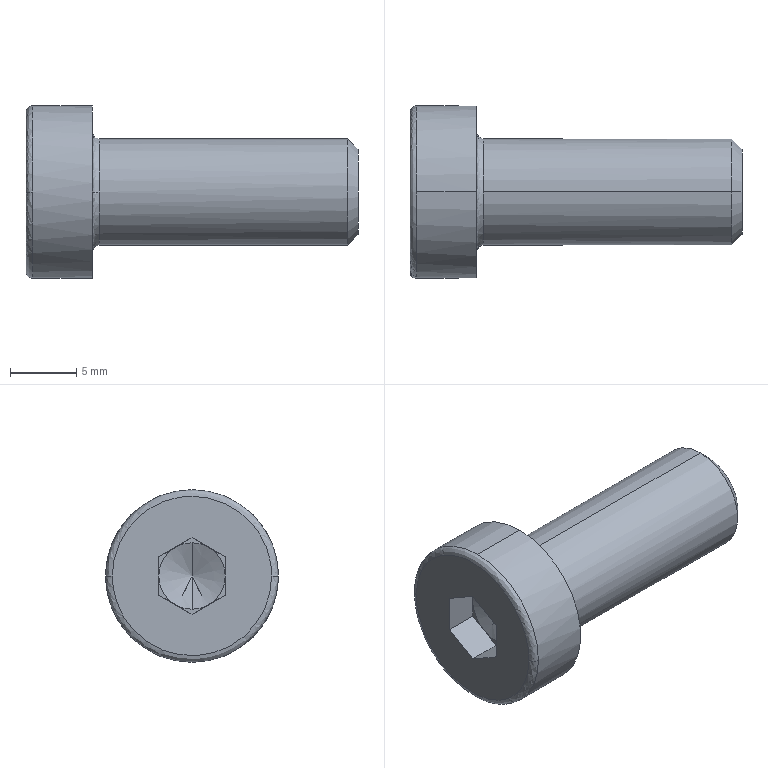Part | SolidWorks | features BaseBody 1 | 1 solid | 27 faces | box 25 x 13 x 13 mm | volume 1601 mm3 | plane 15 | spline 4 | cylinder 4 | cone 4 | commonest cylinder face diameters 8 x2 13 x2
STEP:
#1=CARTESIAN_POINT('',(-16.5,4.,0.));
#2=VERTEX_POINT('',#1);
#3=CARTESIAN_POINT('',(-16.5,0.,4.));
#4=VERTEX_POINT('',#3);
#5=CARTESIAN_POINT('',(-16.5,0.,0.));
#6=DIRECTION('',(1.,0.,0.));
#7=DIRECTION('',(0.,0.,-1.));
#8=AXIS2_PLACEMENT_3D('',#5,#6,#7);
#9=CIRCLE('',#8,4.);
#10=EDGE_CURVE('',#2,#4,#9,.T.);
#11=ORIENTED_EDGE('',*,*,#10,.F.);
#12=CARTESIAN_POINT('',(-17.,4.5,0.));
#13=VERTEX_POINT('',#12);
#14=CARTESIAN_POINT('',(-16.5,4.5,0.));
#15=DIRECTION('',(0.,0.,-1.));
#16=DIRECTION('',(0.,1.,0.));
#17=AXIS2_PLACEMENT_3D('',#14,#15,#16);
#18=CIRCLE('',#17,0.5);
#19=EDGE_CURVE('',#2,#13,#18,.T.);
#20=ORIENTED_EDGE('',*,*,#19,.T.);
#21=CARTESIAN_POINT('',(-17.,0.,4.5));
#22=VERTEX_POINT('',#21);
#23=CARTESIAN_POINT('',(-17.,0.,4.5));
#24=CARTESIAN_POINT('',(-17.,0.286,4.5));
#25=CARTESIAN_POINT('',(-17.,0.7076,4.461));
#26=CARTESIAN_POINT('',(-17.,1.186,4.345));
#27=CARTESIAN_POINT('',(-17.,1.422,4.27));
#28=CARTESIAN_POINT('',(-17.,1.523,4.235));
#29=CARTESIAN_POINT('',(-17.,1.59,4.21));
#30=CARTESIAN_POINT('',(-17.,1.621,4.198));
#31=CARTESIAN_POINT('',(-17.,1.798,4.128));
#32=CARTESIAN_POINT('',(-17.,2.004,4.034));
#33=CARTESIAN_POINT('',(-17.,2.203,3.925));
#34=CARTESIAN_POINT('',(-17.,2.334,3.848));
#35=CARTESIAN_POINT('',(-17.,2.398,3.809));
#36=CARTESIAN_POINT('',(-17.,2.722,3.597));
#37=CARTESIAN_POINT('',(-17.,2.963,3.401));
#38=CARTESIAN_POINT('',(-17.,3.292,3.072));
#39=CARTESIAN_POINT('',(-17.,3.447,2.9));
#40=CARTESIAN_POINT('',(-17.,3.589,2.716));
#41=CARTESIAN_POINT('',(-17.,3.68,2.591));
#42=CARTESIAN_POINT('',(-17.,3.725,2.526));
#43=CARTESIAN_POINT('',(-17.,3.85,2.335));
#44=CARTESIAN_POINT('',(-17.,3.964,2.139));
#45=CARTESIAN_POINT('',(-17.,4.08,1.901));
#46=CARTESIAN_POINT('',(-17.,4.134,1.779));
#47=CARTESIAN_POINT('',(-17.,4.155,1.727));
#48=CARTESIAN_POINT('',(-17.,4.17,1.692));
#49=CARTESIAN_POINT('',(-17.,4.177,1.673));
#50=CARTESIAN_POINT('',(-17.,4.395,1.125));
#51=CARTESIAN_POINT('',(-17.,4.5,0.5724));
#52=CARTESIAN_POINT('',(-17.,4.5,0.));
#53=B_SPLINE_CURVE_WITH_KNOTS('',3,(#23,#24,#25,#26,#27,#28,#29,#30,#31,#32,#33,#34,#35,#36,#37,#38,#39,#40,#41,#42,#43,#44,#45,#46,#47,#48,#49,#50,#51,#52),.UNSPECIFIED.,.F.,.F.,(4,1,1,1,2,2,1,2,2,2,1,2,2,1,1,1,2,2,4),(0.,0.125,0.1875,0.2187,0.2344,0.25,0.3125,0.3438,0.375,0.5,0.5625,0.5938,0.625,0.6875,0.7188,0.7344,0.7422,0.75,1.),.UNSPECIFIED.);
#54=EDGE_CURVE('',#22,#13,#53,.T.);
#55=ORIENTED_EDGE('',*,*,#54,.F.);
#56=CARTESIAN_POINT('',(-17.,-4.5,0.));
#57=VERTEX_POINT('',#56);
#58=CARTESIAN_POINT('',(-17.,-4.5,0.));
#59=CARTESIAN_POINT('',(-17.,-4.5,0.286));
#60=CARTESIAN_POINT('',(-17.,-4.461,0.7076));
#61=CARTESIAN_POINT('',(-17.,-4.345,1.186));
#62=CARTESIAN_POINT('',(-17.,-4.27,1.422));
#63=CARTESIAN_POINT('',(-17.,-4.235,1.523));
#64=CARTESIAN_POINT('',(-17.,-4.21,1.59));
#65=CARTESIAN_POINT('',(-17.,-4.198,1.621));
#66=CARTESIAN_POINT('',(-17.,-4.128,1.798));
#67=CARTESIAN_POINT('',(-17.,-4.034,2.004));
#68=CARTESIAN_POINT('',(-17.,-3.925,2.203));
#69=CARTESIAN_POINT('',(-17.,-3.848,2.334));
#70=CARTESIAN_POINT('',(-17.,-3.809,2.398));
#71=CARTESIAN_POINT('',(-17.,-3.597,2.722));
#72=CARTESIAN_POINT('',(-17.,-3.401,2.963));
#73=CARTESIAN_POINT('',(-17.,-3.072,3.292));
#74=CARTESIAN_POINT('',(-17.,-2.9,3.447));
#75=CARTESIAN_POINT('',(-17.,-2.716,3.589));
#76=CARTESIAN_POINT('',(-17.,-2.591,3.68));
#77=CARTESIAN_POINT('',(-17.,-2.526,3.725));
#78=CARTESIAN_POINT('',(-17.,-2.335,3.85));
#79=CARTESIAN_POINT('',(-17.,-2.139,3.964));
#80=CARTESIAN_POINT('',(-17.,-1.901,4.08));
#81=CARTESIAN_POINT('',(-17.,-1.779,4.134));
#82=CARTESIAN_POINT('',(-17.,-1.727,4.155));
#83=CARTESIAN_POINT('',(-17.,-1.692,4.17));
#84=CARTESIAN_POINT('',(-17.,-1.673,4.177));
#85=CARTESIAN_POINT('',(-17.,-1.125,4.395));
#86=CARTESIAN_POINT('',(-17.,-0.5724,4.5));
#87=CARTESIAN_POINT('',(-17.,0.,4.5));
#88=B_SPLINE_CURVE_WITH_KNOTS('',3,(#58,#59,#60,#61,#62,#63,#64,#65,#66,#67,#68,#69,#70,#71,#72,#73,#74,#75,#76,#77,#78,#79,#80,#81,#82,#83,#84,#85,#86,#87),.UNSPECIFIED.,.F.,.F.,(4,1,1,1,2,2,1,2,2,2,1,2,2,1,1,1,2,2,4),(0.,0.125,0.1875,0.2188,0.2344,0.25,0.3125,0.3438,0.375,0.5,0.5625,0.5938,0.625,0.6875,0.7188,0.7344,0.7422,0.75,1.),.UNSPECIFIED.);
#89=EDGE_CURVE('',#57,#22,#88,.T.);
#90=ORIENTED_EDGE('',*,*,#89,.F.);
#91=CARTESIAN_POINT('',(-16.5,-4.,0.));
#92=VERTEX_POINT('',#91);
#93=CARTESIAN_POINT('',(-16.5,-4.5,0.));
#94=DIRECTION('',(0.,0.,1.));
#95=DIRECTION('',(0.,-1.,0.));
#96=AXIS2_PLACEMENT_3D('',#93,#94,#95);
#97=CIRCLE('',#96,0.5);
#98=EDGE_CURVE('',#92,#57,#97,.T.);
#99=ORIENTED_EDGE('',*,*,#98,.F.);
#100=CARTESIAN_POINT('',(-16.5,0.,0.));
#101=DIRECTION('',(1.,0.,0.));
#102=DIRECTION('',(0.,0.,-1.));
#103=AXIS2_PLACEMENT_3D('',#100,#101,#102);
#104=CIRCLE('',#103,4.);
#105=EDGE_CURVE('',#4,#92,#104,.T.);
#106=ORIENTED_EDGE('',*,*,#105,.F.);
#107=EDGE_LOOP('',(#11,#20,#55,#90,#99,#106));
#108=FACE_OUTER_BOUND('',#107,.T.);
#109=CARTESIAN_POINT('',(-16.5,-4.,0.));
#110=CARTESIAN_POINT('',(-16.5,-4.,8.));
#111=CARTESIAN_POINT('',(-16.5,4.,8.));
#112=CARTESIAN_POINT('',(-16.5,4.,0.));
#113=CARTESIAN_POINT('',(-16.793,-4.,0.));
#114=CARTESIAN_POINT('',(-16.793,-4.,8.));
#115=CARTESIAN_POINT('',(-16.793,4.,8.));
#116=CARTESIAN_POINT('',(-16.793,4.,0.));
#117=CARTESIAN_POINT('',(-17.,-4.207,0.));
#118=CARTESIAN_POINT('',(-17.,-4.207,8.414));
#119=CARTESIAN_POINT('',(-17.,4.207,8.414));
#120=CARTESIAN_POINT('',(-17.,4.207,0.));
#121=CARTESIAN_POINT('',(-17.,-4.5,0.));
#122=CARTESIAN_POINT('',(-17.,-4.5,9.));
#123=CARTESIAN_POINT('',(-17.,4.5,9.));
#124=CARTESIAN_POINT('',(-17.,4.5,0.));
#125=(BOUNDED_SURFACE()B_SPLINE_SURFACE(3,3,((#109,#110,#111,#112),(#113,#114,#115,#116),(#117,#118,#119,#120),(#121,#122,#123,#124)),.UNSPECIFIED.,.F.,.F.,.T.)B_SPLINE_SURFACE_WITH_KNOTS((4,4),(4,4),(0.,1.),(0.,1.),.UNSPECIFIED.)GEOMETRIC_REPRESENTATION_ITEM()RATIONAL_B_SPLINE_SURFACE(((1.,0.3333,0.3333,1.),(0.8047,0.2682,0.2682,0.8047),(0.8047,0.2682,0.2682,0.8047),(1.,0.3333,0.3333,1.)))REPRESENTATION_ITEM('')SURFACE());
#126=ADVANCED_FACE('',(#108),#125,.F.);
#127=CARTESIAN_POINT('',(-22.,-6.,0.));
#128=VERTEX_POINT('',#127);
#129=CARTESIAN_POINT('',(-22.,6.,0.));
#130=VERTEX_POINT('',#129);
#131=CARTESIAN_POINT('',(-22.,-6.,0.));
#132=CARTESIAN_POINT('',(-22.,-6.,-12.));
#133=CARTESIAN_POINT('',(-22.,6.,-12.));
#134=CARTESIAN_POINT('',(-22.,6.,0.));
#135=(BOUNDED_CURVE()B_SPLINE_CURVE(3,(#131,#132,#133,#134),.UNSPECIFIED.,.F.,.T.)B_SPLINE_CURVE_WITH_KNOTS((4,4),(0.,1.),.UNSPECIFIED.)CURVE()GEOMETRIC_REPRESENTATION_ITEM()RATIONAL_B_SPLINE_CURVE((1.,0.3333,0.3333,1.))REPRESENTATION_ITEM(''));
#136=EDGE_CURVE('',#128,#130,#135,.T.);
#137=ORIENTED_EDGE('',*,*,#136,.T.);
#138=CARTESIAN_POINT('',(-21.5,6.5,0.));
#139=VERTEX_POINT('',#138);
#140=CARTESIAN_POINT('',(-21.5,6.,0.));
#141=DIRECTION('',(0.,0.,-1.));
#142=DIRECTION('',(0.,1.,0.));
#143=AXIS2_PLACEMENT_3D('',#140,#141,#142);
#144=CIRCLE('',#143,0.5);
#145=EDGE_CURVE('',#130,#139,#144,.T.);
#146=ORIENTED_EDGE('',*,*,#145,.T.);
#147=CARTESIAN_POINT('',(-21.5,0.,-6.5));
#148=VERTEX_POINT('',#147);
#149=CARTESIAN_POINT('',(-21.5,0.,0.));
#150=DIRECTION('',(1.,0.,0.));
#151=DIRECTION('',(0.,0.,-1.));
#152=AXIS2_PLACEMENT_3D('',#149,#150,#151);
#153=CIRCLE('',#152,6.5);
#154=EDGE_CURVE('',#148,#139,#153,.T.);
#155=ORIENTED_EDGE('',*,*,#154,.F.);
#156=CARTESIAN_POINT('',(-21.5,-6.5,0.));
#157=VERTEX_POINT('',#156);
#158=CARTESIAN_POINT('',(-21.5,0.,0.));
#159=DIRECTION('',(1.,0.,0.));
#160=DIRECTION('',(0.,0.,-1.));
#161=AXIS2_PLACEMENT_3D('',#158,#159,#160);
#162=CIRCLE('',#161,6.5);
#163=EDGE_CURVE('',#157,#148,#162,.T.);
#164=ORIENTED_EDGE('',*,*,#163,.F.);
#165=CARTESIAN_POINT('',(-21.5,-6.,0.));
#166=DIRECTION('',(0.,0.,1.));
#167=DIRECTION('',(0.,-1.,0.));
#168=AXIS2_PLACEMENT_3D('',#165,#166,#167);
#169=CIRCLE('',#168,0.5);
#170=EDGE_CURVE('',#128,#157,#169,.T.);
#171=ORIENTED_EDGE('',*,*,#170,.F.);
#172=EDGE_LOOP('',(#137,#146,#155,#164,#171));
#173=FACE_OUTER_BOUND('',#172,.T.);
#174=CARTESIAN_POINT('',(-22.,6.,0.));
#175=CARTESIAN_POINT('',(-22.,6.,-12.));
#176=CARTESIAN_POINT('',(-22.,-6.,-12.));
#177=CARTESIAN_POINT('',(-22.,-6.,0.));
#178=CARTESIAN_POINT('',(-22.,6.293,0.));
#179=CARTESIAN_POINT('',(-22.,6.293,-12.586));
#180=CARTESIAN_POINT('',(-22.,-6.293,-12.586));
#181=CARTESIAN_POINT('',(-22.,-6.293,0.));
#182=CARTESIAN_POINT('',(-21.793,6.5,0.));
#183=CARTESIAN_POINT('',(-21.793,6.5,-13.));
#184=CARTESIAN_POINT('',(-21.793,-6.5,-13.));
#185=CARTESIAN_POINT('',(-21.793,-6.5,0.));
#186=CARTESIAN_POINT('',(-21.5,6.5,0.));
#187=CARTESIAN_POINT('',(-21.5,6.5,-13.));
#188=CARTESIAN_POINT('',(-21.5,-6.5,-13.));
#189=CARTESIAN_POINT('',(-21.5,-6.5,0.));
#190=(BOUNDED_SURFACE()B_SPLINE_SURFACE(3,3,((#174,#175,#176,#177),(#178,#179,#180,#181),(#182,#183,#184,#185),(#186,#187,#188,#189)),.UNSPECIFIED.,.F.,.F.,.F.)B_SPLINE_SURFACE_WITH_KNOTS((4,4),(4,4),(0.,1.),(0.,1.),.UNSPECIFIED.)GEOMETRIC_REPRESENTATION_ITEM()RATIONAL_B_SPLINE_SURFACE(((1.,0.3333,0.3333,1.),(0.8047,0.2682,0.2682,0.8047),(0.8047,0.2682,0.2682,0.8047),(1.,0.3333,0.3333,1.)))REPRESENTATION_ITEM('')SURFACE());
#191=ADVANCED_FACE('',(#173),#190,.T.);
#192=CARTESIAN_POINT('',(-16.5,0.,-4.));
#193=VERTEX_POINT('',#192);
#194=CARTESIAN_POINT('',(-16.5,0.,0.));
#195=DIRECTION('',(1.,0.,0.));
#196=DIRECTION('',(0.,0.,-1.));
#197=AXIS2_PLACEMENT_3D('',#194,#195,#196);
#198=CIRCLE('',#197,4.);
#199=EDGE_CURVE('',#193,#2,#198,.T.);
#200=ORIENTED_EDGE('',*,*,#199,.T.);
#201=ORIENTED_EDGE('',*,*,#10,.T.);
#202=CARTESIAN_POINT('',(2.233,0.,4.));
#203=VERTEX_POINT('',#202);
#204=CARTESIAN_POINT('',(-7.133,0.,4.));
#205=DIRECTION('',(1.,0.,0.));
#206=VECTOR('',#205,1000.);
#207=LINE('',#204,#206);
#208=EDGE_CURVE('',#4,#203,#207,.T.);
#209=ORIENTED_EDGE('',*,*,#208,.T.);
#210=CARTESIAN_POINT('',(2.233,0.,-4.));
#211=VERTEX_POINT('',#210);
#212=CARTESIAN_POINT('',(2.233,0.,0.));
#213=DIRECTION('',(-1.,0.,0.));
#214=DIRECTION('',(0.,0.,-1.));
#215=AXIS2_PLACEMENT_3D('',#212,#213,#214);
#216=CIRCLE('',#215,4.);
#217=EDGE_CURVE('',#203,#211,#216,.T.);
#218=ORIENTED_EDGE('',*,*,#217,.T.);
#219=CARTESIAN_POINT('',(-7.133,0.,-4.));
#220=DIRECTION('',(1.,0.,0.));
#221=VECTOR('',#220,1000.);
#222=LINE('',#219,#221);
#223=EDGE_CURVE('',#193,#211,#222,.T.);
#224=ORIENTED_EDGE('',*,*,#223,.F.);
#225=EDGE_LOOP('',(#200,#201,#209,#218,#224));
#226=FACE_OUTER_BOUND('',#225,.T.);
#227=CARTESIAN_POINT('',(-7.133,0.,0.));
#228=DIRECTION('',(1.,0.,0.));
#229=DIRECTION('',(0.,0.,-1.));
#230=AXIS2_PLACEMENT_3D('',#227,#228,#229);
#231=CYLINDRICAL_SURFACE('',#230,4.);
#232=ADVANCED_FACE('',(#226),#231,.T.);
#233=CARTESIAN_POINT('',(3.,0.,3.233));
#234=VERTEX_POINT('',#233);
#235=CARTESIAN_POINT('',(3.,0.,-3.233));
#236=VERTEX_POINT('',#235);
#237=CARTESIAN_POINT('',(3.,0.,0.));
#238=DIRECTION('',(-1.,0.,0.));
#239=DIRECTION('',(0.,0.,1.));
#240=AXIS2_PLACEMENT_3D('',#237,#238,#239);
#241=CIRCLE('',#240,3.233);
#242=EDGE_CURVE('',#234,#236,#241,.T.);
#243=ORIENTED_EDGE('',*,*,#242,.T.);
#244=CARTESIAN_POINT('',(2.233,0.,-4.));
#245=DIRECTION('',(-0.7071,0.,-0.7071));
#246=VECTOR('',#245,1000.);
#247=LINE('',#244,#246);
#248=EDGE_CURVE('',#236,#211,#247,.T.);
#249=ORIENTED_EDGE('',*,*,#248,.T.);
#250=ORIENTED_EDGE('',*,*,#217,.F.);
#251=CARTESIAN_POINT('',(2.233,0.,4.));
#252=DIRECTION('',(-0.7071,0.,0.7071));
#253=VECTOR('',#252,1000.);
#254=LINE('',#251,#253);
#255=EDGE_CURVE('',#234,#203,#254,.T.);
#256=ORIENTED_EDGE('',*,*,#255,.F.);
#257=EDGE_LOOP('',(#243,#249,#250,#256));
#258=FACE_OUTER_BOUND('',#257,.T.);
#259=CARTESIAN_POINT('',(2.233,0.,0.));
#260=DIRECTION('',(-1.,0.,0.));
#261=DIRECTION('',(0.,0.,1.));
#262=AXIS2_PLACEMENT_3D('',#259,#260,#261);
#263=CONICAL_SURFACE('',#262,4.,0.7854);
#264=ADVANCED_FACE('',(#258),#263,.T.);
#265=ORIENTED_EDGE('',*,*,#154,.T.);
#266=CARTESIAN_POINT('',(-21.5,0.,6.5));
#267=VERTEX_POINT('',#266);
#268=CARTESIAN_POINT('',(-21.5,0.,0.));
#269=DIRECTION('',(1.,0.,0.));
#270=DIRECTION('',(0.,0.,-1.));
#271=AXIS2_PLACEMENT_3D('',#268,#269,#270);
#272=CIRCLE('',#271,6.5);
#273=EDGE_CURVE('',#139,#267,#272,.T.);
#274=ORIENTED_EDGE('',*,*,#273,.T.);
#275=CARTESIAN_POINT('',(-17.,0.,6.5));
#276=VERTEX_POINT('',#275);
#277=CARTESIAN_POINT('',(-19.25,0.,6.5));
#278=DIRECTION('',(1.,0.,0.));
#279=VECTOR('',#278,1000.);
#280=LINE('',#277,#279);
#281=EDGE_CURVE('',#267,#276,#280,.T.);
#282=ORIENTED_EDGE('',*,*,#281,.T.);
#283=CARTESIAN_POINT('',(-17.,0.,-6.5));
#284=VERTEX_POINT('',#283);
#285=CARTESIAN_POINT('',(-17.,0.,0.));
#286=DIRECTION('',(1.,0.,0.));
#287=DIRECTION('',(0.,0.,-1.));
#288=AXIS2_PLACEMENT_3D('',#285,#286,#287);
#289=CIRCLE('',#288,6.5);
#290=EDGE_CURVE('',#284,#276,#289,.T.);
#291=ORIENTED_EDGE('',*,*,#290,.F.);
#292=CARTESIAN_POINT('',(-19.25,0.,-6.5));
#293=DIRECTION('',(1.,0.,0.));
#294=VECTOR('',#293,1000.);
#295=LINE('',#292,#294);
#296=EDGE_CURVE('',#148,#284,#295,.T.);
#297=ORIENTED_EDGE('',*,*,#296,.F.);
#298=EDGE_LOOP('',(#265,#274,#282,#291,#297));
#299=FACE_OUTER_BOUND('',#298,.T.);
#300=CARTESIAN_POINT('',(-19.25,0.,0.));
#301=DIRECTION('',(1.,0.,0.));
#302=DIRECTION('',(0.,0.,-1.));
#303=AXIS2_PLACEMENT_3D('',#300,#301,#302);
#304=CYLINDRICAL_SURFACE('',#303,6.5);
#305=ADVANCED_FACE('',(#299),#304,.T.);
#306=CARTESIAN_POINT('',(-18.5,0.,0.));
#307=VERTEX_POINT('',#306);
#308=CARTESIAN_POINT('',(-19.5,0.,2.5));
#309=VERTEX_POINT('',#308);
#310=CARTESIAN_POINT('',(-19.5,0.,2.5));
#311=DIRECTION('',(-0.3714,0.,0.9285));
#312=VECTOR('',#311,1000.);
#313=LINE('',#310,#312);
#314=EDGE_CURVE('',#307,#309,#313,.T.);
#315=ORIENTED_EDGE('',*,*,#314,.F.);
#316=CARTESIAN_POINT('',(-19.5,0.,-2.5));
#317=VERTEX_POINT('',#316);
#318=CARTESIAN_POINT('',(-19.5,0.,-2.5));
#319=DIRECTION('',(-0.3714,0.,-0.9285));
#320=VECTOR('',#319,1000.);
#321=LINE('',#318,#320);
#322=EDGE_CURVE('',#307,#317,#321,.T.);
#323=ORIENTED_EDGE('',*,*,#322,.T.);
#324=CARTESIAN_POINT('',(-19.5,-1.25,-2.165));
#325=VERTEX_POINT('',#324);
#326=CARTESIAN_POINT('',(-19.5,0.,0.));
#327=DIRECTION('',(1.,0.,0.));
#328=DIRECTION('',(0.,0.,1.));
#329=AXIS2_PLACEMENT_3D('',#326,#327,#328);
#330=CIRCLE('',#329,2.5);
#331=EDGE_CURVE('',#325,#317,#330,.T.);
#332=ORIENTED_EDGE('',*,*,#331,.F.);
#333=CARTESIAN_POINT('',(-19.5,-2.5,0.));
#334=VERTEX_POINT('',#333);
#335=CARTESIAN_POINT('',(-19.5,0.,0.));
#336=DIRECTION('',(-1.,0.,0.));
#337=DIRECTION('',(0.,0.,1.));
#338=AXIS2_PLACEMENT_3D('',#335,#336,#337);
#339=CIRCLE('',#338,2.5);
#340=EDGE_CURVE('',#325,#334,#339,.T.);
#341=ORIENTED_EDGE('',*,*,#340,.T.);
#342=CARTESIAN_POINT('',(-19.5,-1.25,2.165));
#343=VERTEX_POINT('',#342);
#344=CARTESIAN_POINT('',(-19.5,0.,0.));
#345=DIRECTION('',(1.,0.,0.));
#346=DIRECTION('',(0.,0.,1.));
#347=AXIS2_PLACEMENT_3D('',#344,#345,#346);
#348=CIRCLE('',#347,2.5);
#349=EDGE_CURVE('',#343,#334,#348,.T.);
#350=ORIENTED_EDGE('',*,*,#349,.F.);
#351=CARTESIAN_POINT('',(-19.5,0.,0.));
#352=DIRECTION('',(1.,0.,0.));
#353=DIRECTION('',(0.,0.,1.));
#354=AXIS2_PLACEMENT_3D('',#351,#352,#353);
#355=CIRCLE('',#354,2.5);
#356=EDGE_CURVE('',#309,#343,#355,.T.);
#357=ORIENTED_EDGE('',*,*,#356,.F.);
#358=EDGE_LOOP('',(#315,#323,#332,#341,#350,#357));
#359=FACE_OUTER_BOUND('',#358,.T.);
#360=CARTESIAN_POINT('',(-19.5,0.,0.));
#361=DIRECTION('',(-1.,0.,0.));
#362=DIRECTION('',(0.,0.,1.));
#363=AXIS2_PLACEMENT_3D('',#360,#361,#362);
#364=CONICAL_SURFACE('',#363,2.5,1.19);
#365=ADVANCED_FACE('',(#359),#364,.F.);
#366=ORIENTED_EDGE('',*,*,#208,.F.);
#367=ORIENTED_EDGE('',*,*,#105,.T.);
#368=CARTESIAN_POINT('',(-16.5,0.,0.));
#369=DIRECTION('',(1.,0.,0.));
#370=DIRECTION('',(0.,0.,-1.));
#371=AXIS2_PLACEMENT_3D('',#368,#369,#370);
#372=CIRCLE('',#371,4.);
#373=EDGE_CURVE('',#92,#193,#372,.T.);
#374=ORIENTED_EDGE('',*,*,#373,.T.);
#375=ORIENTED_EDGE('',*,*,#223,.T.);
#376=CARTESIAN_POINT('',(2.233,0.,0.));
#377=DIRECTION('',(-1.,0.,0.));
#378=DIRECTION('',(0.,0.,-1.));
#379=AXIS2_PLACEMENT_3D('',#376,#377,#378);
#380=CIRCLE('',#379,4.);
#381=EDGE_CURVE('',#211,#203,#380,.T.);
#382=ORIENTED_EDGE('',*,*,#381,.T.);
#383=EDGE_LOOP('',(#366,#367,#374,#375,#382));
#384=FACE_OUTER_BOUND('',#383,.T.);
#385=CARTESIAN_POINT('',(-7.133,0.,0.));
#386=DIRECTION('',(1.,0.,0.));
#387=DIRECTION('',(0.,0.,-1.));
#388=AXIS2_PLACEMENT_3D('',#385,#386,#387);
#389=CYLINDRICAL_SURFACE('',#388,4.);
#390=ADVANCED_FACE('',(#384),#389,.T.);
#391=ORIENTED_EDGE('',*,*,#19,.F.);
#392=ORIENTED_EDGE('',*,*,#199,.F.);
#393=ORIENTED_EDGE('',*,*,#373,.F.);
#394=ORIENTED_EDGE('',*,*,#98,.T.);
#395=CARTESIAN_POINT('',(-17.,4.5,0.));
#396=CARTESIAN_POINT('',(-17.,4.5,-0.286));
#397=CARTESIAN_POINT('',(-17.,4.461,-0.7076));
#398=CARTESIAN_POINT('',(-17.,4.345,-1.186));
#399=CARTESIAN_POINT('',(-17.,4.27,-1.422));
#400=CARTESIAN_POINT('',(-17.,4.235,-1.523));
#401=CARTESIAN_POINT('',(-17.,4.21,-1.59));
#402=CARTESIAN_POINT('',(-17.,4.198,-1.621));
#403=CARTESIAN_POINT('',(-17.,4.128,-1.798));
#404=CARTESIAN_POINT('',(-17.,4.034,-2.004));
#405=CARTESIAN_POINT('',(-17.,3.925,-2.203));
#406=CARTESIAN_POINT('',(-17.,3.848,-2.334));
#407=CARTESIAN_POINT('',(-17.,3.809,-2.398));
#408=CARTESIAN_POINT('',(-17.,3.597,-2.722));
#409=CARTESIAN_POINT('',(-17.,3.401,-2.963));
#410=CARTESIAN_POINT('',(-17.,3.072,-3.292));
#411=CARTESIAN_POINT('',(-17.,2.9,-3.447));
#412=CARTESIAN_POINT('',(-17.,2.716,-3.589));
#413=CARTESIAN_POINT('',(-17.,2.591,-3.68));
#414=CARTESIAN_POINT('',(-17.,2.526,-3.725));
#415=CARTESIAN_POINT('',(-17.,2.335,-3.85));
#416=CARTESIAN_POINT('',(-17.,2.139,-3.964));
#417=CARTESIAN_POINT('',(-17.,1.901,-4.08));
#418=CARTESIAN_POINT('',(-17.,1.779,-4.134));
#419=CARTESIAN_POINT('',(-17.,1.727,-4.155));
#420=CARTESIAN_POINT('',(-17.,1.692,-4.17));
#421=CARTESIAN_POINT('',(-17.,1.673,-4.177));
#422=CARTESIAN_POINT('',(-17.,1.125,-4.395));
#423=CARTESIAN_POINT('',(-17.,0.5719,-4.5));
#424=CARTESIAN_POINT('',(-17.,-0.2859,-4.5));
#425=CARTESIAN_POINT('',(-17.,-0.7075,-4.461));
#426=CARTESIAN_POINT('',(-17.,-1.186,-4.345));
#427=CARTESIAN_POINT('',(-17.,-1.422,-4.27));
#428=CARTESIAN_POINT('',(-17.,-1.523,-4.235));
#429=CARTESIAN_POINT('',(-17.,-1.59,-4.21));
#430=CARTESIAN_POINT('',(-17.,-1.621,-4.198));
#431=CARTESIAN_POINT('',(-17.,-1.798,-4.128));
#432=CARTESIAN_POINT('',(-17.,-2.004,-4.034));
#433=CARTESIAN_POINT('',(-17.,-2.203,-3.925));
#434=CARTESIAN_POINT('',(-17.,-2.334,-3.848));
#435=CARTESIAN_POINT('',(-17.,-2.398,-3.809));
#436=CARTESIAN_POINT('',(-17.,-2.722,-3.597));
#437=CARTESIAN_POINT('',(-17.,-2.963,-3.401));
#438=CARTESIAN_POINT('',(-17.,-3.292,-3.072));
#439=CARTESIAN_POINT('',(-17.,-3.447,-2.9));
#440=CARTESIAN_POINT('',(-17.,-3.589,-2.716));
#441=CARTESIAN_POINT('',(-17.,-3.68,-2.591));
#442=CARTESIAN_POINT('',(-17.,-3.725,-2.526));
#443=CARTESIAN_POINT('',(-17.,-3.85,-2.335));
#444=CARTESIAN_POINT('',(-17.,-3.964,-2.139));
#445=CARTESIAN_POINT('',(-17.,-4.08,-1.901));
#446=CARTESIAN_POINT('',(-17.,-4.134,-1.779));
#447=CARTESIAN_POINT('',(-17.,-4.155,-1.727));
#448=CARTESIAN_POINT('',(-17.,-4.17,-1.692));
#449=CARTESIAN_POINT('',(-17.,-4.177,-1.673));
#450=CARTESIAN_POINT('',(-17.,-4.395,-1.125));
#451=CARTESIAN_POINT('',(-17.,-4.5,-0.5724));
#452=CARTESIAN_POINT('',(-17.,-4.5,0.));
#453=B_SPLINE_CURVE_WITH_KNOTS('',3,(#395,#396,#397,#398,#399,#400,#401,#402,#403,#404,#405,#406,#407,#408,#409,#410,#411,#412,#413,#414,#415,#416,#417,#418,#419,#420,#421,#422,#423,#424,#425,#426,#427,#428,#429,#430,#431,#432,#433,#434,#435,#436,#437,#438,#439,#440,#441,#442,#443,#444,#445,#446,#447,#448,#449,#450,#451,#452),.UNSPECIFIED.,.F.,.F.,(4,1,1,1,2,2,1,2,2,2,1,2,2,1,1,1,2,2,2,1,1,1,2,2,1,2,2,2,1,2,2,1,1,1,2,2,4),(0.,0.0625,0.09375,0.1094,0.1172,0.125,0.1562,0.1719,0.1875,0.25,0.2812,0.2969,0.3125,0.3437,0.3594,0.3672,0.3711,0.375,0.5,0.5625,0.5937,0.6094,0.6172,0.625,0.6562,0.6719,0.6875,0.75,0.7813,0.7969,0.8125,0.8438,0.8594,0.8672,0.8711,0.875,1.),.UNSPECIFIED.);
#454=EDGE_CURVE('',#13,#57,#453,.T.);
#455=ORIENTED_EDGE('',*,*,#454,.F.);
#456=EDGE_LOOP('',(#391,#392,#393,#394,#455));
#457=FACE_OUTER_BOUND('',#456,.T.);
#458=CARTESIAN_POINT('',(-16.5,4.,0.));
#459=CARTESIAN_POINT('',(-16.5,4.,-8.));
#460=CARTESIAN_POINT('',(-16.5,-4.,-8.));
#461=CARTESIAN_POINT('',(-16.5,-4.,0.));
#462=CARTESIAN_POINT('',(-16.793,4.,0.));
#463=CARTESIAN_POINT('',(-16.793,4.,-8.));
#464=CARTESIAN_POINT('',(-16.793,-4.,-8.));
#465=CARTESIAN_POINT('',(-16.793,-4.,0.));
#466=CARTESIAN_POINT('',(-17.,4.207,0.));
#467=CARTESIAN_POINT('',(-17.,4.207,-8.414));
#468=CARTESIAN_POINT('',(-17.,-4.207,-8.414));
#469=CARTESIAN_POINT('',(-17.,-4.207,0.));
#470=CARTESIAN_POINT('',(-17.,4.5,0.));
#471=CARTESIAN_POINT('',(-17.,4.5,-9.));
#472=CARTESIAN_POINT('',(-17.,-4.5,-9.));
#473=CARTESIAN_POINT('',(-17.,-4.5,0.));
#474=(BOUNDED_SURFACE()B_SPLINE_SURFACE(3,3,((#458,#459,#460,#461),(#462,#463,#464,#465),(#466,#467,#468,#469),(#470,#471,#472,#473)),.UNSPECIFIED.,.F.,.F.,.T.)B_SPLINE_SURFACE_WITH_KNOTS((4,4),(4,4),(0.,1.),(0.,1.),.UNSPECIFIED.)GEOMETRIC_REPRESENTATION_ITEM()RATIONAL_B_SPLINE_SURFACE(((1.,0.3333,0.3333,1.),(0.8047,0.2682,0.2682,0.8047),(0.8047,0.2682,0.2682,0.8047),(1.,0.3333,0.3333,1.)))REPRESENTATION_ITEM('')SURFACE());
#475=ADVANCED_FACE('',(#457),#474,.F.);
#476=ORIENTED_EDGE('',*,*,#248,.F.);
#477=CARTESIAN_POINT('',(3.,0.,0.));
#478=DIRECTION('',(-1.,0.,0.));
#479=DIRECTION('',(0.,0.,1.));
#480=AXIS2_PLACEMENT_3D('',#477,#478,#479);
#481=CIRCLE('',#480,3.233);
#482=EDGE_CURVE('',#236,#234,#481,.T.);
#483=ORIENTED_EDGE('',*,*,#482,.T.);
#484=ORIENTED_EDGE('',*,*,#255,.T.);
#485=ORIENTED_EDGE('',*,*,#381,.F.);
#486=EDGE_LOOP('',(#476,#483,#484,#485));
#487=FACE_OUTER_BOUND('',#486,.T.);
#488=CARTESIAN_POINT('',(2.233,0.,0.));
#489=DIRECTION('',(-1.,0.,0.));
#490=DIRECTION('',(0.,0.,1.));
#491=AXIS2_PLACEMENT_3D('',#488,#489,#490);
#492=CONICAL_SURFACE('',#491,4.,0.7854);
#493=ADVANCED_FACE('',(#487),#492,.T.);
#494=ORIENTED_EDGE('',*,*,#454,.T.);
#495=ORIENTED_EDGE('',*,*,#89,.T.);
#496=ORIENTED_EDGE('',*,*,#54,.T.);
#497=EDGE_LOOP('',(#494,#495,#496));
#498=FACE_BOUND('',#497,.T.);
#499=ORIENTED_EDGE('',*,*,#290,.T.);
#500=CARTESIAN_POINT('',(-17.,0.,0.));
#501=DIRECTION('',(1.,0.,0.));
#502=DIRECTION('',(0.,0.,-1.));
#503=AXIS2_PLACEMENT_3D('',#500,#501,#502);
#504=CIRCLE('',#503,6.5);
#505=EDGE_CURVE('',#276,#284,#504,.T.);
#506=ORIENTED_EDGE('',*,*,#505,.T.);
#507=EDGE_LOOP('',(#499,#506));
#508=FACE_OUTER_BOUND('',#507,.T.);
#509=CARTESIAN_POINT('',(-17.,0.,5.5));
#510=DIRECTION('',(1.,0.,0.));
#511=DIRECTION('',(0.,0.,-1.));
#512=AXIS2_PLACEMENT_3D('',#509,#510,#511);
#513=PLANE('',#512);
#514=ADVANCED_FACE('',(#498,#508),#513,.T.);
#515=ORIENTED_EDGE('',*,*,#242,.F.);
#516=ORIENTED_EDGE('',*,*,#482,.F.);
#517=EDGE_LOOP('',(#515,#516));
#518=FACE_OUTER_BOUND('',#517,.T.);
#519=CARTESIAN_POINT('',(3.,0.,1.617));
#520=DIRECTION('',(1.,0.,0.));
#521=DIRECTION('',(0.,0.,-1.));
#522=AXIS2_PLACEMENT_3D('',#519,#520,#521);
#523=PLANE('',#522);
#524=ADVANCED_FACE('',(#518),#523,.T.);
#525=ORIENTED_EDGE('',*,*,#281,.F.);
#526=CARTESIAN_POINT('',(-21.5,0.,0.));
#527=DIRECTION('',(1.,0.,0.));
#528=DIRECTION('',(0.,0.,-1.));
#529=AXIS2_PLACEMENT_3D('',#526,#527,#528);
#530=CIRCLE('',#529,6.5);
#531=EDGE_CURVE('',#267,#157,#530,.T.);
#532=ORIENTED_EDGE('',*,*,#531,.T.);
#533=ORIENTED_EDGE('',*,*,#163,.T.);
#534=ORIENTED_EDGE('',*,*,#296,.T.);
#535=ORIENTED_EDGE('',*,*,#505,.F.);
#536=EDGE_LOOP('',(#525,#532,#533,#534,#535));
#537=FACE_OUTER_BOUND('',#536,.T.);
#538=CARTESIAN_POINT('',(-19.25,0.,0.));
#539=DIRECTION('',(1.,0.,0.));
#540=DIRECTION('',(0.,0.,-1.));
#541=AXIS2_PLACEMENT_3D('',#538,#539,#540);
#542=CYLINDRICAL_SURFACE('',#541,6.5);
#543=ADVANCED_FACE('',(#537),#542,.T.);
#544=ORIENTED_EDGE('',*,*,#145,.F.);
#545=CARTESIAN_POINT('',(-22.,0.,6.));
#546=VERTEX_POINT('',#545);
#547=CARTESIAN_POINT('',(-22.,6.,0.));
#548=CARTESIAN_POINT('',(-22.,6.,3.515));
#549=CARTESIAN_POINT('',(-22.,3.515,6.));
#550=CARTESIAN_POINT('',(-22.,0.,6.));
#551=(BOUNDED_CURVE()B_SPLINE_CURVE(3,(#547,#548,#549,#550),.UNSPECIFIED.,.F.,.F.)B_SPLINE_CURVE_WITH_KNOTS((4,4),(0.,1.),.UNSPECIFIED.)CURVE()GEOMETRIC_REPRESENTATION_ITEM()RATIONAL_B_SPLINE_CURVE((1.,0.8047,0.8047,1.))REPRESENTATION_ITEM(''));
#552=EDGE_CURVE('',#130,#546,#551,.T.);
#553=ORIENTED_EDGE('',*,*,#552,.T.);
#554=CARTESIAN_POINT('',(-22.,0.,6.));
#555=CARTESIAN_POINT('',(-22.,-3.515,6.));
#556=CARTESIAN_POINT('',(-22.,-6.,3.515));
#557=CARTESIAN_POINT('',(-22.,-6.,0.));
#558=(BOUNDED_CURVE()B_SPLINE_CURVE(3,(#554,#555,#556,#557),.UNSPECIFIED.,.F.,.F.)B_SPLINE_CURVE_WITH_KNOTS((4,4),(0.,1.),.UNSPECIFIED.)CURVE()GEOMETRIC_REPRESENTATION_ITEM()RATIONAL_B_SPLINE_CURVE((1.,0.8047,0.8047,1.))REPRESENTATION_ITEM(''));
#559=EDGE_CURVE('',#546,#128,#558,.T.);
#560=ORIENTED_EDGE('',*,*,#559,.T.);
#561=ORIENTED_EDGE('',*,*,#170,.T.);
#562=ORIENTED_EDGE('',*,*,#531,.F.);
#563=ORIENTED_EDGE('',*,*,#273,.F.);
#564=EDGE_LOOP('',(#544,#553,#560,#561,#562,#563));
#565=FACE_OUTER_BOUND('',#564,.T.);
#566=CARTESIAN_POINT('',(-22.,-6.,0.));
#567=CARTESIAN_POINT('',(-22.,-6.,12.));
#568=CARTESIAN_POINT('',(-22.,6.,12.));
#569=CARTESIAN_POINT('',(-22.,6.,0.));
#570=CARTESIAN_POINT('',(-22.,-6.293,0.));
#571=CARTESIAN_POINT('',(-22.,-6.293,12.586));
#572=CARTESIAN_POINT('',(-22.,6.293,12.586));
#573=CARTESIAN_POINT('',(-22.,6.293,0.));
#574=CARTESIAN_POINT('',(-21.793,-6.5,0.));
#575=CARTESIAN_POINT('',(-21.793,-6.5,13.));
#576=CARTESIAN_POINT('',(-21.793,6.5,13.));
#577=CARTESIAN_POINT('',(-21.793,6.5,0.));
#578=CARTESIAN_POINT('',(-21.5,-6.5,0.));
#579=CARTESIAN_POINT('',(-21.5,-6.5,13.));
#580=CARTESIAN_POINT('',(-21.5,6.5,13.));
#581=CARTESIAN_POINT('',(-21.5,6.5,0.));
#582=(BOUNDED_SURFACE()B_SPLINE_SURFACE(3,3,((#566,#567,#568,#569),(#570,#571,#572,#573),(#574,#575,#576,#577),(#578,#579,#580,#581)),.UNSPECIFIED.,.F.,.F.,.F.)B_SPLINE_SURFACE_WITH_KNOTS((4,4),(4,4),(0.,1.),(0.,1.),.UNSPECIFIED.)GEOMETRIC_REPRESENTATION_ITEM()RATIONAL_B_SPLINE_SURFACE(((1.,0.3333,0.3333,1.),(0.8047,0.2682,0.2682,0.8047),(0.8047,0.2682,0.2682,0.8047),(1.,0.3333,0.3333,1.)))REPRESENTATION_ITEM('')SURFACE());
#583=ADVANCED_FACE('',(#565),#582,.T.);
#584=ORIENTED_EDGE('',*,*,#136,.F.);
#585=ORIENTED_EDGE('',*,*,#559,.F.);
#586=ORIENTED_EDGE('',*,*,#552,.F.);
#587=EDGE_LOOP('',(#584,#585,#586));
#588=FACE_OUTER_BOUND('',#587,.T.);
#589=CARTESIAN_POINT('',(-22.,2.5,1.443));
#590=VERTEX_POINT('',#589);
#591=CARTESIAN_POINT('',(-22.,0.,2.887));
#592=VERTEX_POINT('',#591);
#593=CARTESIAN_POINT('',(-22.,2.5,1.443));
#594=DIRECTION('',(0.,-0.866,0.5));
#595=VECTOR('',#594,1000.);
#596=LINE('',#593,#595);
#597=EDGE_CURVE('',#590,#592,#596,.T.);
#598=ORIENTED_EDGE('',*,*,#597,.T.);
#599=CARTESIAN_POINT('',(-22.,-2.5,1.443));
#600=VERTEX_POINT('',#599);
#601=CARTESIAN_POINT('',(-22.,0.,2.887));
#602=DIRECTION('',(0.,-0.866,-0.5));
#603=VECTOR('',#602,1000.);
#604=LINE('',#601,#603);
#605=EDGE_CURVE('',#592,#600,#604,.T.);
#606=ORIENTED_EDGE('',*,*,#605,.T.);
#607=CARTESIAN_POINT('',(-22.,-2.5,-1.443));
#608=VERTEX_POINT('',#607);
#609=CARTESIAN_POINT('',(-22.,-2.5,3.));
#610=DIRECTION('',(0.,0.,-1.));
#611=VECTOR('',#610,1000.);
#612=LINE('',#609,#611);
#613=EDGE_CURVE('',#600,#608,#612,.T.);
#614=ORIENTED_EDGE('',*,*,#613,.T.);
#615=CARTESIAN_POINT('',(-22.,0.,-2.887));
#616=VERTEX_POINT('',#615);
#617=CARTESIAN_POINT('',(-22.,-2.5,-1.443));
#618=DIRECTION('',(0.,0.866,-0.5));
#619=VECTOR('',#618,1000.);
#620=LINE('',#617,#619);
#621=EDGE_CURVE('',#608,#616,#620,.T.);
#622=ORIENTED_EDGE('',*,*,#621,.T.);
#623=CARTESIAN_POINT('',(-22.,2.5,-1.443));
#624=VERTEX_POINT('',#623);
#625=CARTESIAN_POINT('',(-22.,0.,-2.887));
#626=DIRECTION('',(0.,0.866,0.5));
#627=VECTOR('',#626,1000.);
#628=LINE('',#625,#627);
#629=EDGE_CURVE('',#616,#624,#628,.T.);
#630=ORIENTED_EDGE('',*,*,#629,.T.);
#631=CARTESIAN_POINT('',(-22.,2.5,3.));
#632=DIRECTION('',(0.,0.,1.));
#633=VECTOR('',#632,1000.);
#634=LINE('',#631,#633);
#635=EDGE_CURVE('',#624,#590,#634,.T.);
#636=ORIENTED_EDGE('',*,*,#635,.T.);
#637=EDGE_LOOP('',(#598,#606,#614,#622,#630,#636));
#638=FACE_BOUND('',#637,.T.);
#639=CARTESIAN_POINT('',(-22.,0.,3.));
#640=DIRECTION('',(-1.,0.,0.));
#641=DIRECTION('',(0.,0.,1.));
#642=AXIS2_PLACEMENT_3D('',#639,#640,#641);
#643=PLANE('',#642);
#644=ADVANCED_FACE('',(#588,#638),#643,.T.);
#645=CARTESIAN_POINT('',(-19.5,0.,2.887));
#646=VERTEX_POINT('',#645);
#647=CARTESIAN_POINT('',(-22.,0.,2.887));
#648=DIRECTION('',(-1.,0.,0.));
#649=VECTOR('',#648,1000.);
#650=LINE('',#647,#649);
#651=EDGE_CURVE('',#646,#592,#650,.T.);
#652=ORIENTED_EDGE('',*,*,#651,.F.);
#653=CARTESIAN_POINT('',(-19.5,-2.5,1.443));
#654=DIRECTION('',(0.,0.866,0.5));
#655=VECTOR('',#654,1000.);
#656=LINE('',#653,#655);
#657=EDGE_CURVE('',#343,#646,#656,.T.);
#658=ORIENTED_EDGE('',*,*,#657,.F.);
#659=CARTESIAN_POINT('',(-19.5,-2.5,1.443));
#660=VERTEX_POINT('',#659);
#661=CARTESIAN_POINT('',(-19.5,-1.25,2.165));
#662=DIRECTION('',(0.,-0.866,-0.5));
#663=VECTOR('',#662,1000.);
#664=LINE('',#661,#663);
#665=EDGE_CURVE('',#343,#660,#664,.T.);
#666=ORIENTED_EDGE('',*,*,#665,.T.);
#667=CARTESIAN_POINT('',(-22.,-2.5,1.443));
#668=DIRECTION('',(1.,0.,0.));
#669=VECTOR('',#668,1000.);
#670=LINE('',#667,#669);
#671=EDGE_CURVE('',#600,#660,#670,.T.);
#672=ORIENTED_EDGE('',*,*,#671,.F.);
#673=ORIENTED_EDGE('',*,*,#605,.F.);
#674=EDGE_LOOP('',(#652,#658,#666,#672,#673));
#675=FACE_OUTER_BOUND('',#674,.T.);
#676=CARTESIAN_POINT('',(-22.,-2.5,1.443));
#677=DIRECTION('',(0.,-0.5,0.866));
#678=DIRECTION('',(0.,-0.866,-0.5));
#679=AXIS2_PLACEMENT_3D('',#676,#677,#678);
#680=PLANE('',#679);
#681=ADVANCED_FACE('',(#675),#680,.F.);
#682=CARTESIAN_POINT('',(-19.5,2.5,1.443));
#683=VERTEX_POINT('',#682);
#684=CARTESIAN_POINT('',(-22.,2.5,1.443));
#685=DIRECTION('',(-1.,0.,0.));
#686=VECTOR('',#685,1000.);
#687=LINE('',#684,#686);
#688=EDGE_CURVE('',#683,#590,#687,.T.);
#689=ORIENTED_EDGE('',*,*,#688,.F.);
#690=CARTESIAN_POINT('',(-19.5,1.25,2.165));
#691=VERTEX_POINT('',#690);
#692=CARTESIAN_POINT('',(-19.5,2.5,1.443));
#693=DIRECTION('',(0.,-0.866,0.5));
#694=VECTOR('',#693,1000.);
#695=LINE('',#692,#694);
#696=EDGE_CURVE('',#683,#691,#695,.T.);
#697=ORIENTED_EDGE('',*,*,#696,.T.);
#698=CARTESIAN_POINT('',(-19.5,0.,2.887));
#699=DIRECTION('',(0.,0.866,-0.5));
#700=VECTOR('',#699,1000.);
#701=LINE('',#698,#700);
#702=EDGE_CURVE('',#646,#691,#701,.T.);
#703=ORIENTED_EDGE('',*,*,#702,.F.);
#704=ORIENTED_EDGE('',*,*,#651,.T.);
#705=ORIENTED_EDGE('',*,*,#597,.F.);
#706=EDGE_LOOP('',(#689,#697,#703,#704,#705));
#707=FACE_OUTER_BOUND('',#706,.T.);
#708=CARTESIAN_POINT('',(-22.,0.,2.887));
#709=DIRECTION('',(0.,0.5,0.866));
#710=DIRECTION('',(0.,-0.866,0.5));
#711=AXIS2_PLACEMENT_3D('',#708,#709,#710);
#712=PLANE('',#711);
#713=ADVANCED_FACE('',(#707),#712,.F.);
#714=CARTESIAN_POINT('',(-19.5,2.5,-1.443));
#715=VERTEX_POINT('',#714);
#716=CARTESIAN_POINT('',(-22.,2.5,-1.443));
#717=DIRECTION('',(-1.,0.,0.));
#718=VECTOR('',#717,1000.);
#719=LINE('',#716,#718);
#720=EDGE_CURVE('',#715,#624,#719,.T.);
#721=ORIENTED_EDGE('',*,*,#720,.F.);
#722=CARTESIAN_POINT('',(-19.5,2.5,0.));
#723=VERTEX_POINT('',#722);
#724=CARTESIAN_POINT('',(-19.5,2.5,0.));
#725=DIRECTION('',(0.,0.,1.));
#726=VECTOR('',#725,1000.);
#727=LINE('',#724,#726);
#728=EDGE_CURVE('',#715,#723,#727,.T.);
#729=ORIENTED_EDGE('',*,*,#728,.T.);
#730=CARTESIAN_POINT('',(-19.5,2.5,0.));
#731=DIRECTION('',(0.,0.,1.));
#732=VECTOR('',#731,1000.);
#733=LINE('',#730,#732);
#734=EDGE_CURVE('',#723,#683,#733,.T.);
#735=ORIENTED_EDGE('',*,*,#734,.T.);
#736=ORIENTED_EDGE('',*,*,#688,.T.);
#737=ORIENTED_EDGE('',*,*,#635,.F.);
#738=EDGE_LOOP('',(#721,#729,#735,#736,#737));
#739=FACE_OUTER_BOUND('',#738,.T.);
#740=CARTESIAN_POINT('',(-22.,2.5,1.443));
#741=DIRECTION('',(0.,1.,0.));
#742=DIRECTION('',(0.,0.,1.));
#743=AXIS2_PLACEMENT_3D('',#740,#741,#742);
#744=PLANE('',#743);
#745=ADVANCED_FACE('',(#739),#744,.F.);
#746=CARTESIAN_POINT('',(-19.5,0.,-2.887));
#747=VERTEX_POINT('',#746);
#748=CARTESIAN_POINT('',(-22.,0.,-2.887));
#749=DIRECTION('',(-1.,0.,0.));
#750=VECTOR('',#749,1000.);
#751=LINE('',#748,#750);
#752=EDGE_CURVE('',#747,#616,#751,.T.);
#753=ORIENTED_EDGE('',*,*,#752,.F.);
#754=CARTESIAN_POINT('',(-19.5,1.25,-2.165));
#755=VERTEX_POINT('',#754);
#756=CARTESIAN_POINT('',(-19.5,2.5,-1.443));
#757=DIRECTION('',(0.,-0.866,-0.5));
#758=VECTOR('',#757,1000.);
#759=LINE('',#756,#758);
#760=EDGE_CURVE('',#755,#747,#759,.T.);
#761=ORIENTED_EDGE('',*,*,#760,.F.);
#762=CARTESIAN_POINT('',(-19.5,1.25,-2.165));
#763=DIRECTION('',(0.,0.866,0.5));
#764=VECTOR('',#763,1000.);
#765=LINE('',#762,#764);
#766=EDGE_CURVE('',#755,#715,#765,.T.);
#767=ORIENTED_EDGE('',*,*,#766,.T.);
#768=ORIENTED_EDGE('',*,*,#720,.T.);
#769=ORIENTED_EDGE('',*,*,#629,.F.);
#770=EDGE_LOOP('',(#753,#761,#767,#768,#769));
#771=FACE_OUTER_BOUND('',#770,.T.);
#772=CARTESIAN_POINT('',(-22.,2.5,-1.443));
#773=DIRECTION('',(0.,0.5,-0.866));
#774=DIRECTION('',(0.,0.866,0.5));
#775=AXIS2_PLACEMENT_3D('',#772,#773,#774);
#776=PLANE('',#775);
#777=ADVANCED_FACE('',(#771),#776,.F.);
#778=CARTESIAN_POINT('',(-19.5,-2.5,-1.443));
#779=VERTEX_POINT('',#778);
#780=CARTESIAN_POINT('',(-22.,-2.5,-1.443));
#781=DIRECTION('',(-1.,0.,0.));
#782=VECTOR('',#781,1000.);
#783=LINE('',#780,#782);
#784=EDGE_CURVE('',#779,#608,#783,.T.);
#785=ORIENTED_EDGE('',*,*,#784,.F.);
#786=CARTESIAN_POINT('',(-19.5,0.,-2.887));
#787=DIRECTION('',(0.,-0.866,0.5));
#788=VECTOR('',#787,1000.);
#789=LINE('',#786,#788);
#790=EDGE_CURVE('',#325,#779,#789,.T.);
#791=ORIENTED_EDGE('',*,*,#790,.F.);
#792=CARTESIAN_POINT('',(-19.5,0.,-2.887));
#793=DIRECTION('',(0.,-0.866,0.5));
#794=VECTOR('',#793,1000.);
#795=LINE('',#792,#794);
#796=EDGE_CURVE('',#747,#325,#795,.T.);
#797=ORIENTED_EDGE('',*,*,#796,.F.);
#798=ORIENTED_EDGE('',*,*,#752,.T.);
#799=ORIENTED_EDGE('',*,*,#621,.F.);
#800=EDGE_LOOP('',(#785,#791,#797,#798,#799));
#801=FACE_OUTER_BOUND('',#800,.T.);
#802=CARTESIAN_POINT('',(-22.,0.,-2.887));
#803=DIRECTION('',(0.,-0.5,-0.866));
#804=DIRECTION('',(0.,0.866,-0.5));
#805=AXIS2_PLACEMENT_3D('',#802,#803,#804);
#806=PLANE('',#805);
#807=ADVANCED_FACE('',(#801),#806,.F.);
#808=ORIENTED_EDGE('',*,*,#671,.T.);
#809=CARTESIAN_POINT('',(-19.5,-2.5,0.));
#810=DIRECTION('',(0.,0.,-1.));
#811=VECTOR('',#810,1000.);
#812=LINE('',#809,#811);
#813=EDGE_CURVE('',#660,#334,#812,.T.);
#814=ORIENTED_EDGE('',*,*,#813,.T.);
#815=CARTESIAN_POINT('',(-19.5,-2.5,-1.443));
#816=DIRECTION('',(0.,0.,1.));
#817=VECTOR('',#816,1000.);
#818=LINE('',#815,#817);
#819=EDGE_CURVE('',#779,#334,#818,.T.);
#820=ORIENTED_EDGE('',*,*,#819,.F.);
#821=ORIENTED_EDGE('',*,*,#784,.T.);
#822=ORIENTED_EDGE('',*,*,#613,.F.);
#823=EDGE_LOOP('',(#808,#814,#820,#821,#822));
#824=FACE_OUTER_BOUND('',#823,.T.);
#825=CARTESIAN_POINT('',(-22.,-2.5,-1.443));
#826=DIRECTION('',(0.,-1.,0.));
#827=DIRECTION('',(0.,0.,-1.));
#828=AXIS2_PLACEMENT_3D('',#825,#826,#827);
#829=PLANE('',#828);
#830=ADVANCED_FACE('',(#824),#829,.F.);
#831=ORIENTED_EDGE('',*,*,#657,.T.);
#832=ORIENTED_EDGE('',*,*,#702,.T.);
#833=CARTESIAN_POINT('',(-19.5,0.,0.));
#834=DIRECTION('',(1.,0.,0.));
#835=DIRECTION('',(0.,0.,1.));
#836=AXIS2_PLACEMENT_3D('',#833,#834,#835);
#837=CIRCLE('',#836,2.5);
#838=EDGE_CURVE('',#691,#309,#837,.T.);
#839=ORIENTED_EDGE('',*,*,#838,.T.);
#840=ORIENTED_EDGE('',*,*,#356,.T.);
#841=EDGE_LOOP('',(#831,#832,#839,#840));
#842=FACE_OUTER_BOUND('',#841,.T.);
#843=CARTESIAN_POINT('',(-19.5,0.,0.));
#844=DIRECTION('',(1.,0.,0.));
#845=DIRECTION('',(0.,0.,-1.));
#846=AXIS2_PLACEMENT_3D('',#843,#844,#845);
#847=PLANE('',#846);
#848=ADVANCED_FACE('',(#842),#847,.F.);
#849=ORIENTED_EDGE('',*,*,#760,.T.);
#850=ORIENTED_EDGE('',*,*,#796,.T.);
#851=ORIENTED_EDGE('',*,*,#331,.T.);
#852=CARTESIAN_POINT('',(-19.5,0.,0.));
#853=DIRECTION('',(1.,0.,0.));
#854=DIRECTION('',(0.,0.,1.));
#855=AXIS2_PLACEMENT_3D('',#852,#853,#854);
#856=CIRCLE('',#855,2.5);
#857=EDGE_CURVE('',#317,#755,#856,.T.);
#858=ORIENTED_EDGE('',*,*,#857,.T.);
#859=EDGE_LOOP('',(#849,#850,#851,#858));
#860=FACE_OUTER_BOUND('',#859,.T.);
#861=CARTESIAN_POINT('',(-19.5,0.,0.));
#862=DIRECTION('',(1.,0.,0.));
#863=DIRECTION('',(0.,0.,-1.));
#864=AXIS2_PLACEMENT_3D('',#861,#862,#863);
#865=PLANE('',#864);
#866=ADVANCED_FACE('',(#860),#865,.F.);
#867=ORIENTED_EDGE('',*,*,#790,.T.);
#868=ORIENTED_EDGE('',*,*,#819,.T.);
#869=ORIENTED_EDGE('',*,*,#340,.F.);
#870=EDGE_LOOP('',(#867,#868,#869));
#871=FACE_OUTER_BOUND('',#870,.T.);
#872=CARTESIAN_POINT('',(-19.5,0.,0.));
#873=DIRECTION('',(1.,0.,0.));
#874=DIRECTION('',(0.,0.,-1.));
#875=AXIS2_PLACEMENT_3D('',#872,#873,#874);
#876=PLANE('',#875);
#877=ADVANCED_FACE('',(#871),#876,.F.);
#878=ORIENTED_EDGE('',*,*,#322,.F.);
#879=ORIENTED_EDGE('',*,*,#314,.T.);
#880=ORIENTED_EDGE('',*,*,#838,.F.);
#881=CARTESIAN_POINT('',(-19.5,0.,0.));
#882=DIRECTION('',(1.,0.,0.));
#883=DIRECTION('',(0.,0.,1.));
#884=AXIS2_PLACEMENT_3D('',#881,#882,#883);
#885=CIRCLE('',#884,2.5);
#886=EDGE_CURVE('',#723,#691,#885,.T.);
#887=ORIENTED_EDGE('',*,*,#886,.F.);
#888=CARTESIAN_POINT('',(-19.5,0.,0.));
#889=DIRECTION('',(1.,0.,0.));
#890=DIRECTION('',(0.,0.,1.));
#891=AXIS2_PLACEMENT_3D('',#888,#889,#890);
#892=CIRCLE('',#891,2.5);
#893=EDGE_CURVE('',#755,#723,#892,.T.);
#894=ORIENTED_EDGE('',*,*,#893,.F.);
#895=ORIENTED_EDGE('',*,*,#857,.F.);
#896=EDGE_LOOP('',(#878,#879,#880,#887,#894,#895));
#897=FACE_OUTER_BOUND('',#896,.T.);
#898=CARTESIAN_POINT('',(-19.5,0.,0.));
#899=DIRECTION('',(-1.,0.,0.));
#900=DIRECTION('',(0.,0.,1.));
#901=AXIS2_PLACEMENT_3D('',#898,#899,#900);
#902=CONICAL_SURFACE('',#901,2.5,1.19);
#903=ADVANCED_FACE('',(#897),#902,.F.);
#904=ORIENTED_EDGE('',*,*,#813,.F.);
#905=ORIENTED_EDGE('',*,*,#665,.F.);
#906=ORIENTED_EDGE('',*,*,#349,.T.);
#907=EDGE_LOOP('',(#904,#905,#906));
#908=FACE_OUTER_BOUND('',#907,.T.);
#909=CARTESIAN_POINT('',(-19.5,0.,0.));
#910=DIRECTION('',(1.,0.,0.));
#911=DIRECTION('',(0.,0.,-1.));
#912=AXIS2_PLACEMENT_3D('',#909,#910,#911);
#913=PLANE('',#912);
#914=ADVANCED_FACE('',(#908),#913,.F.);
#915=ORIENTED_EDGE('',*,*,#696,.F.);
#916=ORIENTED_EDGE('',*,*,#734,.F.);
#917=ORIENTED_EDGE('',*,*,#886,.T.);
#918=EDGE_LOOP('',(#915,#916,#917));
#919=FACE_OUTER_BOUND('',#918,.T.);
#920=CARTESIAN_POINT('',(-19.5,0.,0.));
#921=DIRECTION('',(1.,0.,0.));
#922=DIRECTION('',(0.,0.,-1.));
#923=AXIS2_PLACEMENT_3D('',#920,#921,#922);
#924=PLANE('',#923);
#925=ADVANCED_FACE('',(#919),#924,.F.);
#926=ORIENTED_EDGE('',*,*,#728,.F.);
#927=ORIENTED_EDGE('',*,*,#766,.F.);
#928=ORIENTED_EDGE('',*,*,#893,.T.);
#929=EDGE_LOOP('',(#926,#927,#928));
#930=FACE_OUTER_BOUND('',#929,.T.);
#931=CARTESIAN_POINT('',(-19.5,0.,0.));
#932=DIRECTION('',(1.,0.,0.));
#933=DIRECTION('',(0.,0.,-1.));
#934=AXIS2_PLACEMENT_3D('',#931,#932,#933);
#935=PLANE('',#934);
#936=ADVANCED_FACE('',(#930),#935,.F.);
#937=CLOSED_SHELL('',(#126,#191,#232,#264,#305,#365,#390,#475,#493,#514,#524,#543,#583,#644,#681,#713,#745,#777,#807,#830,#848,#866,#877,#903,#914,#925,#936));
#938=MANIFOLD_SOLID_BREP('',#937);
#939=CARTESIAN_POINT('',(0.,0.,0.));
#940=DIRECTION('',(0.,0.,1.));
#941=DIRECTION('',(1.,0.,0.));
#942=AXIS2_PLACEMENT_3D('',#939,#940,#941);
#943=(LENGTH_UNIT()NAMED_UNIT(*)SI_UNIT(.MILLI.,.METRE.));
#944=UNCERTAINTY_MEASURE_WITH_UNIT(LENGTH_MEASURE(0.00001),#943,'','');
#945=(NAMED_UNIT(*)PLANE_ANGLE_UNIT()SI_UNIT($,.RADIAN.));
#946=(NAMED_UNIT(*)SI_UNIT($,.STERADIAN.)SOLID_ANGLE_UNIT());
#947=(GEOMETRIC_REPRESENTATION_CONTEXT(3)GLOBAL_UNCERTAINTY_ASSIGNED_CONTEXT((#944))GLOBAL_UNIT_ASSIGNED_CONTEXT((#943,#945,#946))REPRESENTATION_CONTEXT('',''));
#948=ADVANCED_BREP_SHAPE_REPRESENTATION('',(#938,#942),#947);